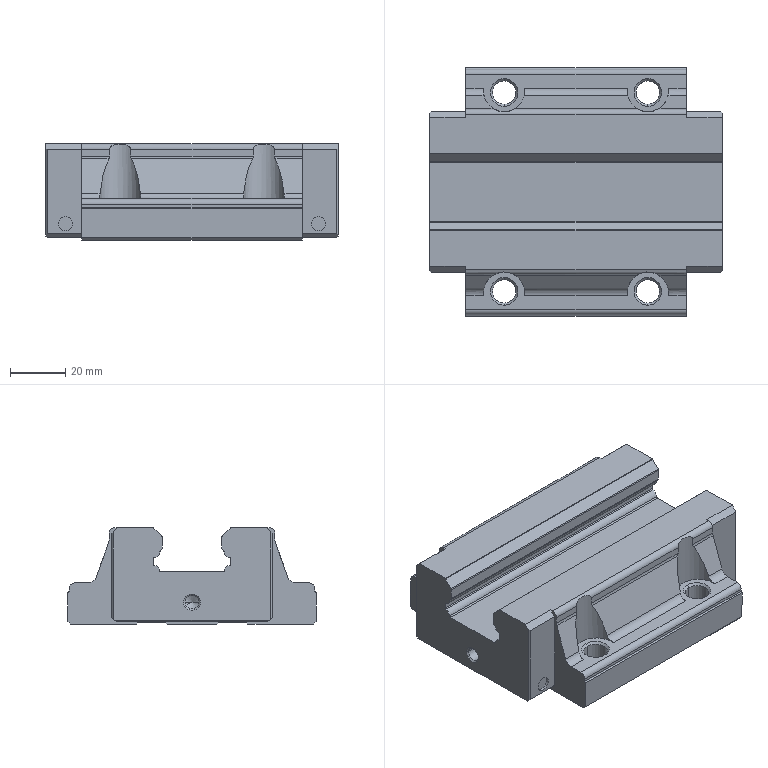Part | STEP file | Moved position-Part-1 | 1 solid | 165 faces | box 106 x 90 x 35 mm | volume 213246 mm3 | plane 76 | cylinder 65 | cone 24 | commonest cylinder face diameters 6 x12 5.2 x8 8.5 x8 15 x6 4 x4 4.917 x4